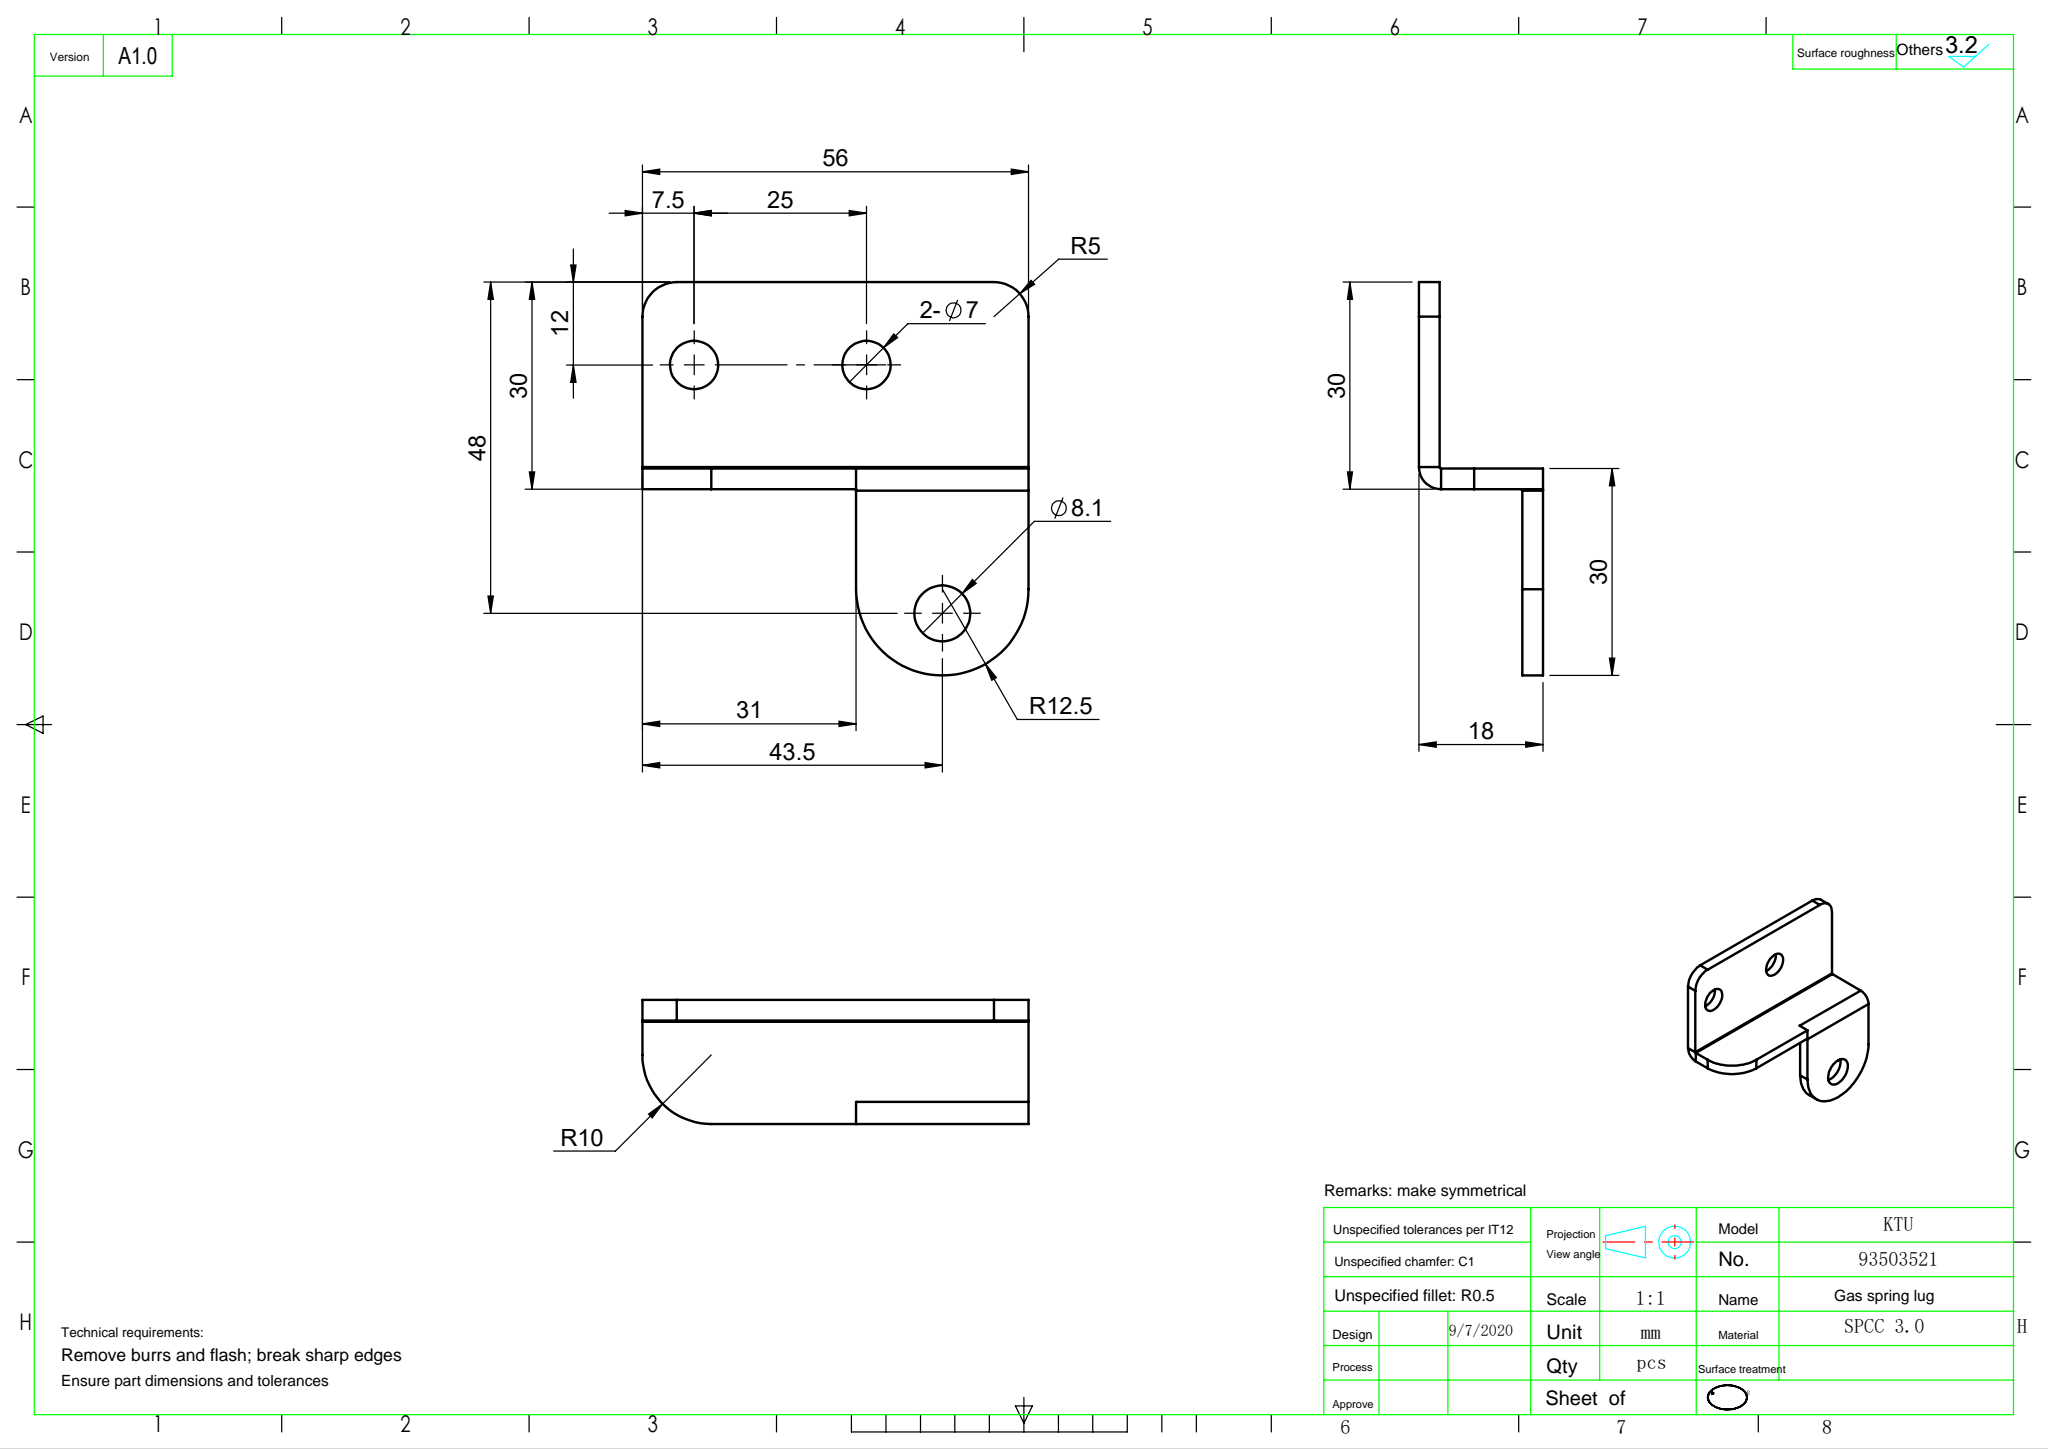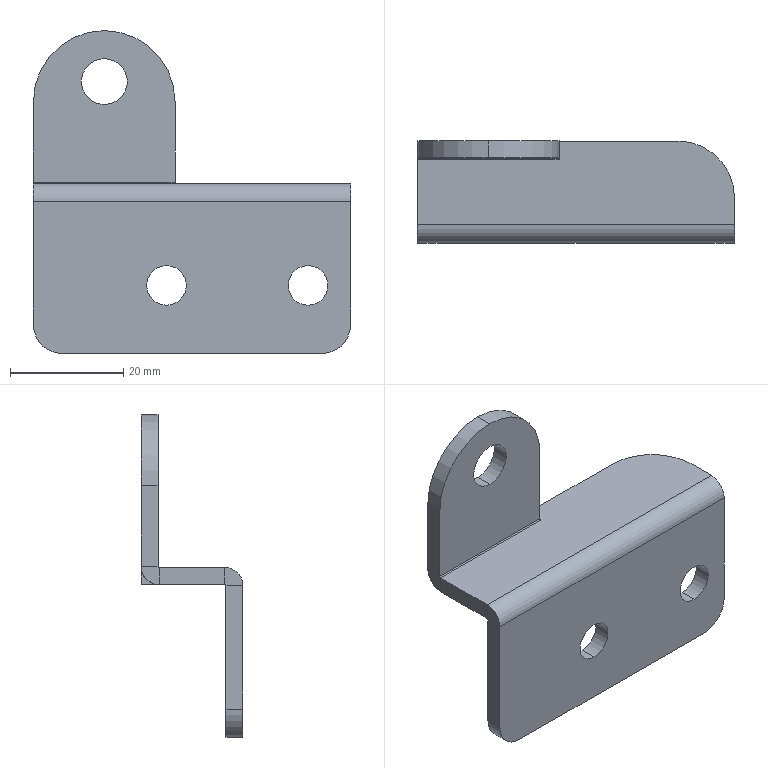Part | SolidWorks | features MirrorStock 1 | 1 solid | 34 faces | box 56 x 18 x 57 mm | volume 8724 mm3 | plane 19 | cylinder 15 | commonest cylinder face diameters 7 x4 0.4 x2 6.4 x2 8.1 x2 10 x2 25 x2
STEP:
#1=CARTESIAN_POINT('',(20.5,-9.,-18.5));
#2=VERTEX_POINT('',#1);
#3=CARTESIAN_POINT('',(20.5,-9.,-11.5));
#4=VERTEX_POINT('',#3);
#5=CARTESIAN_POINT('',(20.5,-9.,-15.));
#6=DIRECTION('',(0.,-1.,0.));
#7=DIRECTION('',(0.,0.,1.));
#8=AXIS2_PLACEMENT_3D('',#5,#6,#7);
#9=CIRCLE('',#8,3.5);
#10=EDGE_CURVE('',#2,#4,#9,.T.);
#11=ORIENTED_EDGE('',*,*,#10,.T.);
#12=CARTESIAN_POINT('',(20.5,-6.,-11.5));
#13=VERTEX_POINT('',#12);
#14=CARTESIAN_POINT('',(20.5,-9.001,-11.5));
#15=DIRECTION('',(0.,1.,0.));
#16=VECTOR('',#15,1000.);
#17=LINE('',#14,#16);
#18=EDGE_CURVE('',#4,#13,#17,.T.);
#19=ORIENTED_EDGE('',*,*,#18,.T.);
#20=CARTESIAN_POINT('',(20.5,-6.,-18.5));
#21=VERTEX_POINT('',#20);
#22=CARTESIAN_POINT('',(20.5,-6.,-15.));
#23=DIRECTION('',(0.,-1.,0.));
#24=DIRECTION('',(0.,0.,-1.));
#25=AXIS2_PLACEMENT_3D('',#22,#23,#24);
#26=CIRCLE('',#25,3.5);
#27=EDGE_CURVE('',#21,#13,#26,.T.);
#28=ORIENTED_EDGE('',*,*,#27,.F.);
#29=CARTESIAN_POINT('',(20.5,-9.001,-18.5));
#30=DIRECTION('',(0.,1.,0.));
#31=VECTOR('',#30,1000.);
#32=LINE('',#29,#31);
#33=EDGE_CURVE('',#2,#21,#32,.T.);
#34=ORIENTED_EDGE('',*,*,#33,.F.);
#35=EDGE_LOOP('',(#11,#19,#28,#34));
#36=FACE_OUTER_BOUND('',#35,.T.);
#37=CARTESIAN_POINT('',(20.5,-9.001,-15.));
#38=DIRECTION('',(0.,1.,0.));
#39=DIRECTION('',(0.,0.,-1.));
#40=AXIS2_PLACEMENT_3D('',#37,#38,#39);
#41=CYLINDRICAL_SURFACE('',#40,3.5);
#42=ADVANCED_FACE('',(#36),#41,.F.);
#43=CARTESIAN_POINT('',(-4.5,-9.,-18.5));
#44=VERTEX_POINT('',#43);
#45=CARTESIAN_POINT('',(-4.5,-9.,-11.5));
#46=VERTEX_POINT('',#45);
#47=CARTESIAN_POINT('',(-4.5,-9.,-15.));
#48=DIRECTION('',(0.,-1.,0.));
#49=DIRECTION('',(0.,0.,1.));
#50=AXIS2_PLACEMENT_3D('',#47,#48,#49);
#51=CIRCLE('',#50,3.5);
#52=EDGE_CURVE('',#44,#46,#51,.T.);
#53=ORIENTED_EDGE('',*,*,#52,.T.);
#54=CARTESIAN_POINT('',(-4.5,-6.,-11.5));
#55=VERTEX_POINT('',#54);
#56=CARTESIAN_POINT('',(-4.5,-9.001,-11.5));
#57=DIRECTION('',(0.,1.,0.));
#58=VECTOR('',#57,1000.);
#59=LINE('',#56,#58);
#60=EDGE_CURVE('',#46,#55,#59,.T.);
#61=ORIENTED_EDGE('',*,*,#60,.T.);
#62=CARTESIAN_POINT('',(-4.5,-6.,-18.5));
#63=VERTEX_POINT('',#62);
#64=CARTESIAN_POINT('',(-4.5,-6.,-15.));
#65=DIRECTION('',(0.,-1.,0.));
#66=DIRECTION('',(0.,0.,-1.));
#67=AXIS2_PLACEMENT_3D('',#64,#65,#66);
#68=CIRCLE('',#67,3.5);
#69=EDGE_CURVE('',#63,#55,#68,.T.);
#70=ORIENTED_EDGE('',*,*,#69,.F.);
#71=CARTESIAN_POINT('',(-4.5,-9.001,-18.5));
#72=DIRECTION('',(0.,1.,0.));
#73=VECTOR('',#72,1000.);
#74=LINE('',#71,#73);
#75=EDGE_CURVE('',#44,#63,#74,.T.);
#76=ORIENTED_EDGE('',*,*,#75,.F.);
#77=EDGE_LOOP('',(#53,#61,#70,#76));
#78=FACE_OUTER_BOUND('',#77,.T.);
#79=CARTESIAN_POINT('',(-4.5,-9.001,-15.));
#80=DIRECTION('',(0.,1.,0.));
#81=DIRECTION('',(0.,0.,-1.));
#82=AXIS2_PLACEMENT_3D('',#79,#80,#81);
#83=CYLINDRICAL_SURFACE('',#82,3.5);
#84=ADVANCED_FACE('',(#78),#83,.F.);
#85=CARTESIAN_POINT('',(-15.5,6.,25.05));
#86=VERTEX_POINT('',#85);
#87=CARTESIAN_POINT('',(-15.5,6.,16.95));
#88=VERTEX_POINT('',#87);
#89=CARTESIAN_POINT('',(-15.5,6.,21.));
#90=DIRECTION('',(0.,1.,0.));
#91=DIRECTION('',(0.,0.,-1.));
#92=AXIS2_PLACEMENT_3D('',#89,#90,#91);
#93=CIRCLE('',#92,4.05);
#94=EDGE_CURVE('',#86,#88,#93,.T.);
#95=ORIENTED_EDGE('',*,*,#94,.F.);
#96=CARTESIAN_POINT('',(-15.5,9.,25.05));
#97=VERTEX_POINT('',#96);
#98=CARTESIAN_POINT('',(-15.5,-9.001,25.05));
#99=DIRECTION('',(0.,1.,0.));
#100=VECTOR('',#99,1000.);
#101=LINE('',#98,#100);
#102=EDGE_CURVE('',#86,#97,#101,.T.);
#103=ORIENTED_EDGE('',*,*,#102,.T.);
#104=CARTESIAN_POINT('',(-15.5,9.,16.95));
#105=VERTEX_POINT('',#104);
#106=CARTESIAN_POINT('',(-15.5,9.,21.));
#107=DIRECTION('',(0.,-1.,0.));
#108=DIRECTION('',(0.,0.,-1.));
#109=AXIS2_PLACEMENT_3D('',#106,#107,#108);
#110=CIRCLE('',#109,4.05);
#111=EDGE_CURVE('',#105,#97,#110,.T.);
#112=ORIENTED_EDGE('',*,*,#111,.F.);
#113=CARTESIAN_POINT('',(-15.5,-9.001,16.95));
#114=DIRECTION('',(0.,1.,0.));
#115=VECTOR('',#114,1000.);
#116=LINE('',#113,#115);
#117=EDGE_CURVE('',#88,#105,#116,.T.);
#118=ORIENTED_EDGE('',*,*,#117,.F.);
#119=EDGE_LOOP('',(#95,#103,#112,#118));
#120=FACE_OUTER_BOUND('',#119,.T.);
#121=CARTESIAN_POINT('',(-15.5,-9.001,21.));
#122=DIRECTION('',(0.,1.,0.));
#123=DIRECTION('',(0.,0.,-1.));
#124=AXIS2_PLACEMENT_3D('',#121,#122,#123);
#125=CYLINDRICAL_SURFACE('',#124,4.05);
#126=ADVANCED_FACE('',(#120),#125,.F.);
#127=CARTESIAN_POINT('',(-3.,9.,17.5));
#128=VERTEX_POINT('',#127);
#129=CARTESIAN_POINT('',(-15.5,9.,30.));
#130=VERTEX_POINT('',#129);
#131=CARTESIAN_POINT('',(-15.5,9.,17.5));
#132=DIRECTION('',(0.,-1.,0.));
#133=DIRECTION('',(0.,0.,-1.));
#134=AXIS2_PLACEMENT_3D('',#131,#132,#133);
#135=CIRCLE('',#134,12.5);
#136=EDGE_CURVE('',#128,#130,#135,.T.);
#137=ORIENTED_EDGE('',*,*,#136,.T.);
#138=CARTESIAN_POINT('',(-15.5,6.,30.));
#139=VERTEX_POINT('',#138);
#140=CARTESIAN_POINT('',(-15.5,6.,30.));
#141=DIRECTION('',(0.,-1.,0.));
#142=VECTOR('',#141,1000.);
#143=LINE('',#140,#142);
#144=EDGE_CURVE('',#130,#139,#143,.T.);
#145=ORIENTED_EDGE('',*,*,#144,.T.);
#146=CARTESIAN_POINT('',(-3.,6.,17.5));
#147=VERTEX_POINT('',#146);
#148=CARTESIAN_POINT('',(-15.5,6.,17.5));
#149=DIRECTION('',(0.,1.,0.));
#150=DIRECTION('',(0.,0.,-1.));
#151=AXIS2_PLACEMENT_3D('',#148,#149,#150);
#152=CIRCLE('',#151,12.5);
#153=EDGE_CURVE('',#139,#147,#152,.T.);
#154=ORIENTED_EDGE('',*,*,#153,.T.);
#155=CARTESIAN_POINT('',(-3.,9.,17.5));
#156=DIRECTION('',(0.,1.,0.));
#157=VECTOR('',#156,1000.);
#158=LINE('',#155,#157);
#159=EDGE_CURVE('',#147,#128,#158,.T.);
#160=ORIENTED_EDGE('',*,*,#159,.T.);
#161=EDGE_LOOP('',(#137,#145,#154,#160));
#162=FACE_OUTER_BOUND('',#161,.T.);
#163=CARTESIAN_POINT('',(-15.5,6.,17.5));
#164=DIRECTION('',(0.,-1.,0.));
#165=DIRECTION('',(0.,0.,1.));
#166=AXIS2_PLACEMENT_3D('',#163,#164,#165);
#167=CYLINDRICAL_SURFACE('',#166,12.5);
#168=ADVANCED_FACE('',(#162),#167,.T.);
#169=ORIENTED_EDGE('',*,*,#144,.F.);
#170=CARTESIAN_POINT('',(-28.,9.,17.5));
#171=VERTEX_POINT('',#170);
#172=CARTESIAN_POINT('',(-15.5,9.,17.5));
#173=DIRECTION('',(0.,-1.,0.));
#174=DIRECTION('',(0.,0.,-1.));
#175=AXIS2_PLACEMENT_3D('',#172,#173,#174);
#176=CIRCLE('',#175,12.5);
#177=EDGE_CURVE('',#130,#171,#176,.T.);
#178=ORIENTED_EDGE('',*,*,#177,.T.);
#179=CARTESIAN_POINT('',(-28.,6.,17.5));
#180=VERTEX_POINT('',#179);
#181=CARTESIAN_POINT('',(-28.,9.,17.5));
#182=DIRECTION('',(0.,-1.,0.));
#183=VECTOR('',#182,1000.);
#184=LINE('',#181,#183);
#185=EDGE_CURVE('',#171,#180,#184,.T.);
#186=ORIENTED_EDGE('',*,*,#185,.T.);
#187=CARTESIAN_POINT('',(-15.5,6.,17.5));
#188=DIRECTION('',(0.,1.,0.));
#189=DIRECTION('',(0.,0.,-1.));
#190=AXIS2_PLACEMENT_3D('',#187,#188,#189);
#191=CIRCLE('',#190,12.5);
#192=EDGE_CURVE('',#180,#139,#191,.T.);
#193=ORIENTED_EDGE('',*,*,#192,.T.);
#194=EDGE_LOOP('',(#169,#178,#186,#193));
#195=FACE_OUTER_BOUND('',#194,.T.);
#196=CARTESIAN_POINT('',(-15.5,6.,17.5));
#197=DIRECTION('',(0.,-1.,0.));
#198=DIRECTION('',(0.,0.,1.));
#199=AXIS2_PLACEMENT_3D('',#196,#197,#198);
#200=CYLINDRICAL_SURFACE('',#199,12.5);
#201=ADVANCED_FACE('',(#195),#200,.T.);
#202=CARTESIAN_POINT('',(-3.,9.,3.));
#203=VERTEX_POINT('',#202);
#204=CARTESIAN_POINT('',(-3.,8.994,3.));
#205=VERTEX_POINT('',#204);
#206=CARTESIAN_POINT('',(-3.,9.,3.));
#207=DIRECTION('',(0.,-1.,0.));
#208=VECTOR('',#207,1000.);
#209=LINE('',#206,#208);
#210=EDGE_CURVE('',#203,#205,#209,.T.);
#211=ORIENTED_EDGE('',*,*,#210,.F.);
#212=CARTESIAN_POINT('',(-3.,9.,0.));
#213=VERTEX_POINT('',#212);
#214=CARTESIAN_POINT('',(-3.,9.,3.));
#215=DIRECTION('',(0.,0.,-1.));
#216=VECTOR('',#215,1000.);
#217=LINE('',#214,#216);
#218=EDGE_CURVE('',#203,#213,#217,.T.);
#219=ORIENTED_EDGE('',*,*,#218,.T.);
#220=CARTESIAN_POINT('',(-3.,5.8,0.));
#221=VERTEX_POINT('',#220);
#222=CARTESIAN_POINT('',(-3.,0.,0.));
#223=DIRECTION('',(0.,-1.,0.));
#224=VECTOR('',#223,1000.);
#225=LINE('',#222,#224);
#226=EDGE_CURVE('',#213,#221,#225,.T.);
#227=ORIENTED_EDGE('',*,*,#226,.T.);
#228=CARTESIAN_POINT('',(-3.,5.8,3.2));
#229=DIRECTION('',(-1.,0.,0.));
#230=DIRECTION('',(0.,0.,1.));
#231=AXIS2_PLACEMENT_3D('',#228,#229,#230);
#232=CIRCLE('',#231,3.2);
#233=EDGE_CURVE('',#205,#221,#232,.T.);
#234=ORIENTED_EDGE('',*,*,#233,.F.);
#235=EDGE_LOOP('',(#211,#219,#227,#234));
#236=FACE_OUTER_BOUND('',#235,.T.);
#237=CARTESIAN_POINT('',(-3.,9.,3.));
#238=DIRECTION('',(-1.,0.,0.));
#239=DIRECTION('',(0.,0.,-1.));
#240=AXIS2_PLACEMENT_3D('',#237,#238,#239);
#241=PLANE('',#240);
#242=ADVANCED_FACE('',(#236),#241,.T.);
#243=CARTESIAN_POINT('',(18.,9.,3.));
#244=VERTEX_POINT('',#243);
#245=CARTESIAN_POINT('',(28.,9.,3.));
#246=DIRECTION('',(-1.,0.,0.));
#247=VECTOR('',#246,1000.);
#248=LINE('',#245,#247);
#249=EDGE_CURVE('',#244,#203,#248,.T.);
#250=ORIENTED_EDGE('',*,*,#249,.T.);
#251=ORIENTED_EDGE('',*,*,#210,.T.);
#252=CARTESIAN_POINT('',(-3.,5.8,3.));
#253=VERTEX_POINT('',#252);
#254=CARTESIAN_POINT('',(-3.,9.,3.));
#255=DIRECTION('',(0.,-1.,0.));
#256=VECTOR('',#255,1000.);
#257=LINE('',#254,#256);
#258=EDGE_CURVE('',#205,#253,#257,.T.);
#259=ORIENTED_EDGE('',*,*,#258,.T.);
#260=CARTESIAN_POINT('',(-28.,5.8,3.));
#261=VERTEX_POINT('',#260);
#262=CARTESIAN_POINT('',(-3.,5.8,3.));
#263=DIRECTION('',(-1.,0.,0.));
#264=VECTOR('',#263,1000.);
#265=LINE('',#262,#264);
#266=EDGE_CURVE('',#253,#261,#265,.T.);
#267=ORIENTED_EDGE('',*,*,#266,.T.);
#268=CARTESIAN_POINT('',(-28.,-5.8,3.));
#269=VERTEX_POINT('',#268);
#270=CARTESIAN_POINT('',(-28.,-9.,3.));
#271=DIRECTION('',(0.,-1.,0.));
#272=VECTOR('',#271,1000.);
#273=LINE('',#270,#272);
#274=EDGE_CURVE('',#261,#269,#273,.T.);
#275=ORIENTED_EDGE('',*,*,#274,.T.);
#276=CARTESIAN_POINT('',(28.,-5.8,3.));
#277=VERTEX_POINT('',#276);
#278=CARTESIAN_POINT('',(28.,-5.8,3.));
#279=DIRECTION('',(-1.,0.,0.));
#280=VECTOR('',#279,1000.);
#281=LINE('',#278,#280);
#282=EDGE_CURVE('',#277,#269,#281,.T.);
#283=ORIENTED_EDGE('',*,*,#282,.F.);
#284=CARTESIAN_POINT('',(28.,-1.,3.));
#285=VERTEX_POINT('',#284);
#286=CARTESIAN_POINT('',(28.,-9.,3.));
#287=DIRECTION('',(0.,1.,0.));
#288=VECTOR('',#287,1000.);
#289=LINE('',#286,#288);
#290=EDGE_CURVE('',#277,#285,#289,.T.);
#291=ORIENTED_EDGE('',*,*,#290,.T.);
#292=CARTESIAN_POINT('',(18.,-1.,3.));
#293=DIRECTION('',(0.,0.,-1.));
#294=DIRECTION('',(1.,0.,0.));
#295=AXIS2_PLACEMENT_3D('',#292,#293,#294);
#296=CIRCLE('',#295,10.);
#297=EDGE_CURVE('',#244,#285,#296,.T.);
#298=ORIENTED_EDGE('',*,*,#297,.F.);
#299=EDGE_LOOP('',(#250,#251,#259,#267,#275,#283,#291,#298));
#300=FACE_OUTER_BOUND('',#299,.T.);
#301=CARTESIAN_POINT('',(0.,0.,3.));
#302=DIRECTION('',(0.,0.,-1.));
#303=DIRECTION('',(1.,0.,0.));
#304=AXIS2_PLACEMENT_3D('',#301,#302,#303);
#305=PLANE('',#304);
#306=ADVANCED_FACE('',(#300),#305,.F.);
#307=CARTESIAN_POINT('',(28.,-5.8,0.));
#308=VERTEX_POINT('',#307);
#309=CARTESIAN_POINT('',(28.,-1.,0.));
#310=VERTEX_POINT('',#309);
#311=CARTESIAN_POINT('',(28.,-9.,0.));
#312=DIRECTION('',(0.,1.,0.));
#313=VECTOR('',#312,1000.);
#314=LINE('',#311,#313);
#315=EDGE_CURVE('',#308,#310,#314,.T.);
#316=ORIENTED_EDGE('',*,*,#315,.F.);
#317=CARTESIAN_POINT('',(-28.,-5.8,0.));
#318=VERTEX_POINT('',#317);
#319=CARTESIAN_POINT('',(28.,-5.8,0.));
#320=DIRECTION('',(-1.,0.,0.));
#321=VECTOR('',#320,1000.);
#322=LINE('',#319,#321);
#323=EDGE_CURVE('',#308,#318,#322,.T.);
#324=ORIENTED_EDGE('',*,*,#323,.T.);
#325=CARTESIAN_POINT('',(-28.,5.8,0.));
#326=VERTEX_POINT('',#325);
#327=CARTESIAN_POINT('',(-28.,-9.,0.));
#328=DIRECTION('',(0.,-1.,0.));
#329=VECTOR('',#328,1000.);
#330=LINE('',#327,#329);
#331=EDGE_CURVE('',#326,#318,#330,.T.);
#332=ORIENTED_EDGE('',*,*,#331,.F.);
#333=CARTESIAN_POINT('',(-3.,5.8,0.));
#334=DIRECTION('',(-1.,0.,0.));
#335=VECTOR('',#334,1000.);
#336=LINE('',#333,#335);
#337=EDGE_CURVE('',#221,#326,#336,.T.);
#338=ORIENTED_EDGE('',*,*,#337,.F.);
#339=ORIENTED_EDGE('',*,*,#226,.F.);
#340=CARTESIAN_POINT('',(18.,9.,0.));
#341=VERTEX_POINT('',#340);
#342=CARTESIAN_POINT('',(28.,9.,0.));
#343=DIRECTION('',(-1.,0.,0.));
#344=VECTOR('',#343,1000.);
#345=LINE('',#342,#344);
#346=EDGE_CURVE('',#341,#213,#345,.T.);
#347=ORIENTED_EDGE('',*,*,#346,.F.);
#348=CARTESIAN_POINT('',(18.,-1.,0.));
#349=DIRECTION('',(0.,0.,1.));
#350=DIRECTION('',(1.,0.,0.));
#351=AXIS2_PLACEMENT_3D('',#348,#349,#350);
#352=CIRCLE('',#351,10.);
#353=EDGE_CURVE('',#310,#341,#352,.T.);
#354=ORIENTED_EDGE('',*,*,#353,.F.);
#355=EDGE_LOOP('',(#316,#324,#332,#338,#339,#347,#354));
#356=FACE_OUTER_BOUND('',#355,.T.);
#357=CARTESIAN_POINT('',(0.,0.,0.));
#358=DIRECTION('',(0.,0.,-1.));
#359=DIRECTION('',(1.,0.,0.));
#360=AXIS2_PLACEMENT_3D('',#357,#358,#359);
#361=PLANE('',#360);
#362=ADVANCED_FACE('',(#356),#361,.T.);
#363=ORIENTED_EDGE('',*,*,#346,.T.);
#364=ORIENTED_EDGE('',*,*,#218,.F.);
#365=ORIENTED_EDGE('',*,*,#249,.F.);
#366=CARTESIAN_POINT('',(18.,9.,3.));
#367=DIRECTION('',(0.,0.,1.));
#368=VECTOR('',#367,1000.);
#369=LINE('',#366,#368);
#370=EDGE_CURVE('',#341,#244,#369,.T.);
#371=ORIENTED_EDGE('',*,*,#370,.F.);
#372=EDGE_LOOP('',(#363,#364,#365,#371));
#373=FACE_OUTER_BOUND('',#372,.T.);
#374=CARTESIAN_POINT('',(28.,9.,3.));
#375=DIRECTION('',(0.,1.,0.));
#376=DIRECTION('',(-1.,0.,0.));
#377=AXIS2_PLACEMENT_3D('',#374,#375,#376);
#378=PLANE('',#377);
#379=ADVANCED_FACE('',(#373),#378,.T.);
#380=ORIENTED_EDGE('',*,*,#290,.F.);
#381=CARTESIAN_POINT('',(28.,-5.8,0.));
#382=DIRECTION('',(0.,0.,1.));
#383=VECTOR('',#382,1000.);
#384=LINE('',#381,#383);
#385=EDGE_CURVE('',#308,#277,#384,.T.);
#386=ORIENTED_EDGE('',*,*,#385,.F.);
#387=ORIENTED_EDGE('',*,*,#315,.T.);
#388=CARTESIAN_POINT('',(28.,-1.,3.));
#389=DIRECTION('',(0.,0.,-1.));
#390=VECTOR('',#389,1000.);
#391=LINE('',#388,#390);
#392=EDGE_CURVE('',#285,#310,#391,.T.);
#393=ORIENTED_EDGE('',*,*,#392,.F.);
#394=EDGE_LOOP('',(#380,#386,#387,#393));
#395=FACE_OUTER_BOUND('',#394,.T.);
#396=CARTESIAN_POINT('',(28.,-9.,3.));
#397=DIRECTION('',(1.,0.,0.));
#398=DIRECTION('',(0.,0.,1.));
#399=AXIS2_PLACEMENT_3D('',#396,#397,#398);
#400=PLANE('',#399);
#401=ADVANCED_FACE('',(#395),#400,.T.);
#402=CARTESIAN_POINT('',(-28.,5.8,3.));
#403=DIRECTION('',(0.,0.,-1.));
#404=VECTOR('',#403,1000.);
#405=LINE('',#402,#404);
#406=EDGE_CURVE('',#261,#326,#405,.T.);
#407=ORIENTED_EDGE('',*,*,#406,.T.);
#408=ORIENTED_EDGE('',*,*,#331,.T.);
#409=CARTESIAN_POINT('',(-28.,-5.8,0.));
#410=DIRECTION('',(0.,0.,1.));
#411=VECTOR('',#410,1000.);
#412=LINE('',#409,#411);
#413=EDGE_CURVE('',#318,#269,#412,.T.);
#414=ORIENTED_EDGE('',*,*,#413,.T.);
#415=ORIENTED_EDGE('',*,*,#274,.F.);
#416=EDGE_LOOP('',(#407,#408,#414,#415));
#417=FACE_OUTER_BOUND('',#416,.T.);
#418=CARTESIAN_POINT('',(-28.,-9.,3.));
#419=DIRECTION('',(-1.,0.,0.));
#420=DIRECTION('',(0.,0.,-1.));
#421=AXIS2_PLACEMENT_3D('',#418,#419,#420);
#422=PLANE('',#421);
#423=ADVANCED_FACE('',(#417),#422,.T.);
#424=CARTESIAN_POINT('',(-28.,-6.,-0.2));
#425=VERTEX_POINT('',#424);
#426=CARTESIAN_POINT('',(-28.,-9.,-0.2));
#427=VERTEX_POINT('',#426);
#428=CARTESIAN_POINT('',(-28.,-9.,-0.2));
#429=DIRECTION('',(0.,-1.,0.));
#430=VECTOR('',#429,1000.);
#431=LINE('',#428,#430);
#432=EDGE_CURVE('',#425,#427,#431,.T.);
#433=ORIENTED_EDGE('',*,*,#432,.T.);
#434=CARTESIAN_POINT('',(-28.,-5.8,-0.2));
#435=DIRECTION('',(1.,0.,0.));
#436=DIRECTION('',(0.,0.,1.));
#437=AXIS2_PLACEMENT_3D('',#434,#435,#436);
#438=CIRCLE('',#437,3.2);
#439=EDGE_CURVE('',#269,#427,#438,.T.);
#440=ORIENTED_EDGE('',*,*,#439,.F.);
#441=ORIENTED_EDGE('',*,*,#413,.F.);
#442=CARTESIAN_POINT('',(-28.,-5.8,-0.2));
#443=DIRECTION('',(1.,0.,0.));
#444=DIRECTION('',(0.,0.,1.));
#445=AXIS2_PLACEMENT_3D('',#442,#443,#444);
#446=CIRCLE('',#445,0.2);
#447=EDGE_CURVE('',#318,#425,#446,.T.);
#448=ORIENTED_EDGE('',*,*,#447,.T.);
#449=EDGE_LOOP('',(#433,#440,#441,#448));
#450=FACE_OUTER_BOUND('',#449,.T.);
#451=CARTESIAN_POINT('',(-28.,-5.8,-0.2));
#452=DIRECTION('',(-1.,0.,0.));
#453=DIRECTION('',(0.,0.,-1.));
#454=AXIS2_PLACEMENT_3D('',#451,#452,#453);
#455=PLANE('',#454);
#456=ADVANCED_FACE('',(#450),#455,.T.);
#457=CARTESIAN_POINT('',(28.,-6.,-0.2));
#458=VERTEX_POINT('',#457);
#459=CARTESIAN_POINT('',(28.,-5.8,-0.2));
#460=DIRECTION('',(-1.,0.,0.));
#461=DIRECTION('',(0.,0.,1.));
#462=AXIS2_PLACEMENT_3D('',#459,#460,#461);
#463=CIRCLE('',#462,0.2);
#464=EDGE_CURVE('',#458,#308,#463,.T.);
#465=ORIENTED_EDGE('',*,*,#464,.T.);
#466=ORIENTED_EDGE('',*,*,#385,.T.);
#467=CARTESIAN_POINT('',(28.,-9.,-0.2));
#468=VERTEX_POINT('',#467);
#469=CARTESIAN_POINT('',(28.,-5.8,-0.2));
#470=DIRECTION('',(-1.,0.,0.));
#471=DIRECTION('',(0.,0.,1.));
#472=AXIS2_PLACEMENT_3D('',#469,#470,#471);
#473=CIRCLE('',#472,3.2);
#474=EDGE_CURVE('',#468,#277,#473,.T.);
#475=ORIENTED_EDGE('',*,*,#474,.F.);
#476=CARTESIAN_POINT('',(28.,-6.,-0.2));
#477=DIRECTION('',(0.,-1.,0.));
#478=VECTOR('',#477,1000.);
#479=LINE('',#476,#478);
#480=EDGE_CURVE('',#458,#468,#479,.T.);
#481=ORIENTED_EDGE('',*,*,#480,.F.);
#482=EDGE_LOOP('',(#465,#466,#475,#481));
#483=FACE_OUTER_BOUND('',#482,.T.);
#484=CARTESIAN_POINT('',(28.,-5.8,-0.2));
#485=DIRECTION('',(-1.,0.,0.));
#486=DIRECTION('',(0.,0.,-1.));
#487=AXIS2_PLACEMENT_3D('',#484,#485,#486);
#488=PLANE('',#487);
#489=ADVANCED_FACE('',(#483),#488,.F.);
#490=ORIENTED_EDGE('',*,*,#282,.T.);
#491=ORIENTED_EDGE('',*,*,#439,.T.);
#492=CARTESIAN_POINT('',(0.,-9.,-0.2));
#493=DIRECTION('',(1.,0.,0.));
#494=VECTOR('',#493,1000.);
#495=LINE('',#492,#494);
#496=EDGE_CURVE('',#427,#468,#495,.T.);
#497=ORIENTED_EDGE('',*,*,#496,.T.);
#498=ORIENTED_EDGE('',*,*,#474,.T.);
#499=EDGE_LOOP('',(#490,#491,#497,#498));
#500=FACE_OUTER_BOUND('',#499,.T.);
#501=CARTESIAN_POINT('',(28.,-5.8,-0.2));
#502=DIRECTION('',(1.,0.,0.));
#503=DIRECTION('',(0.,-1.,0.));
#504=AXIS2_PLACEMENT_3D('',#501,#502,#503);
#505=CYLINDRICAL_SURFACE('',#504,3.2);
#506=ADVANCED_FACE('',(#500),#505,.T.);
#507=ORIENTED_EDGE('',*,*,#323,.F.);
#508=ORIENTED_EDGE('',*,*,#464,.F.);
#509=CARTESIAN_POINT('',(-28.,-6.,-0.2));
#510=DIRECTION('',(1.,0.,0.));
#511=VECTOR('',#510,1000.);
#512=LINE('',#509,#511);
#513=EDGE_CURVE('',#425,#458,#512,.T.);
#514=ORIENTED_EDGE('',*,*,#513,.F.);
#515=ORIENTED_EDGE('',*,*,#447,.F.);
#516=EDGE_LOOP('',(#507,#508,#514,#515));
#517=FACE_OUTER_BOUND('',#516,.T.);
#518=CARTESIAN_POINT('',(28.,-5.8,-0.2));
#519=DIRECTION('',(1.,0.,0.));
#520=DIRECTION('',(0.,-1.,0.));
#521=AXIS2_PLACEMENT_3D('',#518,#519,#520);
#522=CYLINDRICAL_SURFACE('',#521,0.2);
#523=ADVANCED_FACE('',(#517),#522,.F.);
#524=CARTESIAN_POINT('',(28.,-6.,-22.));
#525=VERTEX_POINT('',#524);
#526=CARTESIAN_POINT('',(28.,-6.,0.));
#527=DIRECTION('',(0.,0.,1.));
#528=VECTOR('',#527,1000.);
#529=LINE('',#526,#528);
#530=EDGE_CURVE('',#525,#458,#529,.T.);
#531=ORIENTED_EDGE('',*,*,#530,.T.);
#532=ORIENTED_EDGE('',*,*,#480,.T.);
#533=CARTESIAN_POINT('',(28.,-9.,-22.));
#534=VERTEX_POINT('',#533);
#535=CARTESIAN_POINT('',(28.,-9.,0.));
#536=DIRECTION('',(0.,0.,1.));
#537=VECTOR('',#536,1000.);
#538=LINE('',#535,#537);
#539=EDGE_CURVE('',#534,#468,#538,.T.);
#540=ORIENTED_EDGE('',*,*,#539,.F.);
#541=CARTESIAN_POINT('',(28.,-9.,-22.));
#542=DIRECTION('',(0.,-1.,0.));
#543=VECTOR('',#542,1000.);
#544=LINE('',#541,#543);
#545=EDGE_CURVE('',#525,#534,#544,.T.);
#546=ORIENTED_EDGE('',*,*,#545,.F.);
#547=EDGE_LOOP('',(#531,#532,#540,#546));
#548=FACE_OUTER_BOUND('',#547,.T.);
#549=CARTESIAN_POINT('',(28.,-9.,0.));
#550=DIRECTION('',(1.,0.,0.));
#551=DIRECTION('',(0.,0.,1.));
#552=AXIS2_PLACEMENT_3D('',#549,#550,#551);
#553=PLANE('',#552);
#554=ADVANCED_FACE('',(#548),#553,.T.);
#555=CARTESIAN_POINT('',(-28.,-9.,-22.));
#556=VERTEX_POINT('',#555);
#557=CARTESIAN_POINT('',(-28.,-9.,-27.));
#558=DIRECTION('',(0.,0.,-1.));
#559=VECTOR('',#558,1000.);
#560=LINE('',#557,#559);
#561=EDGE_CURVE('',#427,#556,#560,.T.);
#562=ORIENTED_EDGE('',*,*,#561,.F.);
#563=ORIENTED_EDGE('',*,*,#432,.F.);
#564=CARTESIAN_POINT('',(-28.,-6.,-22.));
#565=VERTEX_POINT('',#564);
#566=CARTESIAN_POINT('',(-28.,-6.,0.));
#567=DIRECTION('',(0.,0.,-1.));
#568=VECTOR('',#567,1000.);
#569=LINE('',#566,#568);
#570=EDGE_CURVE('',#425,#565,#569,.T.);
#571=ORIENTED_EDGE('',*,*,#570,.T.);
#572=CARTESIAN_POINT('',(-28.,-9.,-22.));
#573=DIRECTION('',(0.,1.,0.));
#574=VECTOR('',#573,1000.);
#575=LINE('',#572,#574);
#576=EDGE_CURVE('',#556,#565,#575,.T.);
#577=ORIENTED_EDGE('',*,*,#576,.F.);
#578=EDGE_LOOP('',(#562,#563,#571,#577));
#579=FACE_OUTER_BOUND('',#578,.T.);
#580=CARTESIAN_POINT('',(-28.,-9.,-27.));
#581=DIRECTION('',(-1.,0.,0.));
#582=DIRECTION('',(0.,0.,-1.));
#583=AXIS2_PLACEMENT_3D('',#580,#581,#582);
#584=PLANE('',#583);
#585=ADVANCED_FACE('',(#579),#584,.T.);
#586=ORIENTED_EDGE('',*,*,#10,.F.);
#587=CARTESIAN_POINT('',(20.5,-9.,-15.));
#588=DIRECTION('',(0.,-1.,0.));
#589=DIRECTION('',(0.,0.,1.));
#590=AXIS2_PLACEMENT_3D('',#587,#588,#589);
#591=CIRCLE('',#590,3.5);
#592=EDGE_CURVE('',#4,#2,#591,.T.);
#593=ORIENTED_EDGE('',*,*,#592,.F.);
#594=EDGE_LOOP('',(#586,#593));
#595=FACE_BOUND('',#594,.T.);
#596=ORIENTED_EDGE('',*,*,#52,.F.);
#597=CARTESIAN_POINT('',(-4.5,-9.,-15.));
#598=DIRECTION('',(0.,-1.,0.));
#599=DIRECTION('',(0.,0.,1.));
#600=AXIS2_PLACEMENT_3D('',#597,#598,#599);
#601=CIRCLE('',#600,3.5);
#602=EDGE_CURVE('',#46,#44,#601,.T.);
#603=ORIENTED_EDGE('',*,*,#602,.F.);
#604=EDGE_LOOP('',(#596,#603));
#605=FACE_BOUND('',#604,.T.);
#606=CARTESIAN_POINT('',(-23.,-9.,-27.));
#607=VERTEX_POINT('',#606);
#608=CARTESIAN_POINT('',(23.,-9.,-27.));
#609=VERTEX_POINT('',#608);
#610=CARTESIAN_POINT('',(28.,-9.,-27.));
#611=DIRECTION('',(1.,0.,0.));
#612=VECTOR('',#611,1000.);
#613=LINE('',#610,#612);
#614=EDGE_CURVE('',#607,#609,#613,.T.);
#615=ORIENTED_EDGE('',*,*,#614,.T.);
#616=CARTESIAN_POINT('',(23.,-9.,-22.));
#617=DIRECTION('',(0.,1.,0.));
#618=DIRECTION('',(0.,0.,1.));
#619=AXIS2_PLACEMENT_3D('',#616,#617,#618);
#620=CIRCLE('',#619,5.);
#621=EDGE_CURVE('',#534,#609,#620,.T.);
#622=ORIENTED_EDGE('',*,*,#621,.F.);
#623=ORIENTED_EDGE('',*,*,#539,.T.);
#624=ORIENTED_EDGE('',*,*,#496,.F.);
#625=ORIENTED_EDGE('',*,*,#561,.T.);
#626=CARTESIAN_POINT('',(-23.,-9.,-22.));
#627=DIRECTION('',(0.,1.,0.));
#628=DIRECTION('',(0.,0.,1.));
#629=AXIS2_PLACEMENT_3D('',#626,#627,#628);
#630=CIRCLE('',#629,5.);
#631=EDGE_CURVE('',#607,#556,#630,.T.);
#632=ORIENTED_EDGE('',*,*,#631,.F.);
#633=EDGE_LOOP('',(#615,#622,#623,#624,#625,#632));
#634=FACE_OUTER_BOUND('',#633,.T.);
#635=CARTESIAN_POINT('',(0.,-9.,0.));
#636=DIRECTION('',(0.,-1.,0.));
#637=DIRECTION('',(0.,0.,1.));
#638=AXIS2_PLACEMENT_3D('',#635,#636,#637);
#639=PLANE('',#638);
#640=ADVANCED_FACE('',(#595,#605,#634),#639,.T.);
#641=ORIENTED_EDGE('',*,*,#27,.T.);
#642=CARTESIAN_POINT('',(20.5,-6.,-15.));
#643=DIRECTION('',(0.,-1.,0.));
#644=DIRECTION('',(0.,0.,-1.));
#645=AXIS2_PLACEMENT_3D('',#642,#643,#644);
#646=CIRCLE('',#645,3.5);
#647=EDGE_CURVE('',#13,#21,#646,.T.);
#648=ORIENTED_EDGE('',*,*,#647,.T.);
#649=EDGE_LOOP('',(#641,#648));
#650=FACE_BOUND('',#649,.T.);
#651=ORIENTED_EDGE('',*,*,#69,.T.);
#652=CARTESIAN_POINT('',(-4.5,-6.,-15.));
#653=DIRECTION('',(0.,-1.,0.));
#654=DIRECTION('',(0.,0.,-1.));
#655=AXIS2_PLACEMENT_3D('',#652,#653,#654);
#656=CIRCLE('',#655,3.5);
#657=EDGE_CURVE('',#55,#63,#656,.T.);
#658=ORIENTED_EDGE('',*,*,#657,.T.);
#659=EDGE_LOOP('',(#651,#658));
#660=FACE_BOUND('',#659,.T.);
#661=ORIENTED_EDGE('',*,*,#570,.F.);
#662=ORIENTED_EDGE('',*,*,#513,.T.);
#663=ORIENTED_EDGE('',*,*,#530,.F.);
#664=CARTESIAN_POINT('',(23.,-6.,-27.));
#665=VERTEX_POINT('',#664);
#666=CARTESIAN_POINT('',(23.,-6.,-22.));
#667=DIRECTION('',(0.,-1.,0.));
#668=DIRECTION('',(0.,0.,1.));
#669=AXIS2_PLACEMENT_3D('',#666,#667,#668);
#670=CIRCLE('',#669,5.);
#671=EDGE_CURVE('',#665,#525,#670,.T.);
#672=ORIENTED_EDGE('',*,*,#671,.F.);
#673=CARTESIAN_POINT('',(-23.,-6.,-27.));
#674=VERTEX_POINT('',#673);
#675=CARTESIAN_POINT('',(0.,-6.,-27.));
#676=DIRECTION('',(1.,0.,0.));
#677=VECTOR('',#676,1000.);
#678=LINE('',#675,#677);
#679=EDGE_CURVE('',#674,#665,#678,.T.);
#680=ORIENTED_EDGE('',*,*,#679,.F.);
#681=CARTESIAN_POINT('',(-23.,-6.,-22.));
#682=DIRECTION('',(0.,-1.,0.));
#683=DIRECTION('',(0.,0.,1.));
#684=AXIS2_PLACEMENT_3D('',#681,#682,#683);
#685=CIRCLE('',#684,5.);
#686=EDGE_CURVE('',#565,#674,#685,.T.);
#687=ORIENTED_EDGE('',*,*,#686,.F.);
#688=EDGE_LOOP('',(#661,#662,#663,#672,#680,#687));
#689=FACE_OUTER_BOUND('',#688,.T.);
#690=CARTESIAN_POINT('',(0.,-6.,0.));
#691=DIRECTION('',(0.,-1.,0.));
#692=DIRECTION('',(0.,0.,1.));
#693=AXIS2_PLACEMENT_3D('',#690,#691,#692);
#694=PLANE('',#693);
#695=ADVANCED_FACE('',(#650,#660,#689),#694,.F.);
#696=ORIENTED_EDGE('',*,*,#679,.T.);
#697=CARTESIAN_POINT('',(23.,-9.,-27.));
#698=DIRECTION('',(0.,1.,0.));
#699=VECTOR('',#698,1000.);
#700=LINE('',#697,#699);
#701=EDGE_CURVE('',#609,#665,#700,.T.);
#702=ORIENTED_EDGE('',*,*,#701,.F.);
#703=ORIENTED_EDGE('',*,*,#614,.F.);
#704=CARTESIAN_POINT('',(-23.,-9.,-27.));
#705=DIRECTION('',(0.,-1.,0.));
#706=VECTOR('',#705,1000.);
#707=LINE('',#704,#706);
#708=EDGE_CURVE('',#674,#607,#707,.T.);
#709=ORIENTED_EDGE('',*,*,#708,.F.);
#710=EDGE_LOOP('',(#696,#702,#703,#709));
#711=FACE_OUTER_BOUND('',#710,.T.);
#712=CARTESIAN_POINT('',(28.,-9.,-27.));
#713=DIRECTION('',(0.,0.,-1.));
#714=DIRECTION('',(0.,-1.,0.));
#715=AXIS2_PLACEMENT_3D('',#712,#713,#714);
#716=PLANE('',#715);
#717=ADVANCED_FACE('',(#711),#716,.T.);
#718=CARTESIAN_POINT('',(-28.,6.,3.2));
#719=VERTEX_POINT('',#718);
#720=CARTESIAN_POINT('',(-28.,9.,3.2));
#721=VERTEX_POINT('',#720);
#722=CARTESIAN_POINT('',(-28.,9.,3.2));
#723=DIRECTION('',(0.,1.,0.));
#724=VECTOR('',#723,1000.);
#725=LINE('',#722,#724);
#726=EDGE_CURVE('',#719,#721,#725,.T.);
#727=ORIENTED_EDGE('',*,*,#726,.T.);
#728=CARTESIAN_POINT('',(-28.,5.8,3.2));
#729=DIRECTION('',(1.,0.,0.));
#730=DIRECTION('',(0.,0.,1.));
#731=AXIS2_PLACEMENT_3D('',#728,#729,#730);
#732=CIRCLE('',#731,3.2);
#733=EDGE_CURVE('',#326,#721,#732,.T.);
#734=ORIENTED_EDGE('',*,*,#733,.F.);
#735=ORIENTED_EDGE('',*,*,#406,.F.);
#736=CARTESIAN_POINT('',(-28.,5.8,3.2));
#737=DIRECTION('',(1.,0.,0.));
#738=DIRECTION('',(0.,0.,1.));
#739=AXIS2_PLACEMENT_3D('',#736,#737,#738);
#740=CIRCLE('',#739,0.2);
#741=EDGE_CURVE('',#261,#719,#740,.T.);
#742=ORIENTED_EDGE('',*,*,#741,.T.);
#743=EDGE_LOOP('',(#727,#734,#735,#742));
#744=FACE_OUTER_BOUND('',#743,.T.);
#745=CARTESIAN_POINT('',(-28.,5.8,3.2));
#746=DIRECTION('',(-1.,0.,0.));
#747=DIRECTION('',(0.,0.,-1.));
#748=AXIS2_PLACEMENT_3D('',#745,#746,#747);
#749=PLANE('',#748);
#750=ADVANCED_FACE('',(#744),#749,.T.);
#751=CARTESIAN_POINT('',(-3.,9.,3.2));
#752=VERTEX_POINT('',#751);
#753=CARTESIAN_POINT('',(-3.,5.8,3.2));
#754=DIRECTION('',(-1.,0.,0.));
#755=DIRECTION('',(0.,0.,1.));
#756=AXIS2_PLACEMENT_3D('',#753,#754,#755);
#757=CIRCLE('',#756,3.2);
#758=EDGE_CURVE('',#752,#205,#757,.T.);
#759=ORIENTED_EDGE('',*,*,#758,.F.);
#760=CARTESIAN_POINT('',(-3.,6.,3.2));
#761=VERTEX_POINT('',#760);
#762=CARTESIAN_POINT('',(-3.,6.,3.2));
#763=DIRECTION('',(0.,1.,0.));
#764=VECTOR('',#763,1000.);
#765=LINE('',#762,#764);
#766=EDGE_CURVE('',#761,#752,#765,.T.);
#767=ORIENTED_EDGE('',*,*,#766,.F.);
#768=CARTESIAN_POINT('',(-3.,5.8,3.2));
#769=DIRECTION('',(-1.,0.,0.));
#770=DIRECTION('',(0.,0.,1.));
#771=AXIS2_PLACEMENT_3D('',#768,#769,#770);
#772=CIRCLE('',#771,0.2);
#773=EDGE_CURVE('',#761,#253,#772,.T.);
#774=ORIENTED_EDGE('',*,*,#773,.T.);
#775=ORIENTED_EDGE('',*,*,#258,.F.);
#776=EDGE_LOOP('',(#759,#767,#774,#775));
#777=FACE_OUTER_BOUND('',#776,.T.);
#778=CARTESIAN_POINT('',(-3.,5.8,3.2));
#779=DIRECTION('',(-1.,0.,0.));
#780=DIRECTION('',(0.,0.,-1.));
#781=AXIS2_PLACEMENT_3D('',#778,#779,#780);
#782=PLANE('',#781);
#783=ADVANCED_FACE('',(#777),#782,.F.);
#784=ORIENTED_EDGE('',*,*,#337,.T.);
#785=ORIENTED_EDGE('',*,*,#733,.T.);
#786=CARTESIAN_POINT('',(0.,9.,3.2));
#787=DIRECTION('',(1.,0.,0.));
#788=VECTOR('',#787,1000.);
#789=LINE('',#786,#788);
#790=EDGE_CURVE('',#721,#752,#789,.T.);
#791=ORIENTED_EDGE('',*,*,#790,.T.);
#792=ORIENTED_EDGE('',*,*,#758,.T.);
#793=ORIENTED_EDGE('',*,*,#233,.T.);
#794=EDGE_LOOP('',(#784,#785,#791,#792,#793));
#795=FACE_OUTER_BOUND('',#794,.T.);
#796=CARTESIAN_POINT('',(-3.,5.8,3.2));
#797=DIRECTION('',(1.,0.,0.));
#798=DIRECTION('',(0.,1.,0.));
#799=AXIS2_PLACEMENT_3D('',#796,#797,#798);
#800=CYLINDRICAL_SURFACE('',#799,3.2);
#801=ADVANCED_FACE('',(#795),#800,.T.);
#802=ORIENTED_EDGE('',*,*,#266,.F.);
#803=ORIENTED_EDGE('',*,*,#773,.F.);
#804=CARTESIAN_POINT('',(-28.,6.,3.2));
#805=DIRECTION('',(1.,0.,0.));
#806=VECTOR('',#805,1000.);
#807=LINE('',#804,#806);
#808=EDGE_CURVE('',#719,#761,#807,.T.);
#809=ORIENTED_EDGE('',*,*,#808,.F.);
#810=ORIENTED_EDGE('',*,*,#741,.F.);
#811=EDGE_LOOP('',(#802,#803,#809,#810));
#812=FACE_OUTER_BOUND('',#811,.T.);
#813=CARTESIAN_POINT('',(-3.,5.8,3.2));
#814=DIRECTION('',(1.,0.,0.));
#815=DIRECTION('',(0.,1.,0.));
#816=AXIS2_PLACEMENT_3D('',#813,#814,#815);
#817=CYLINDRICAL_SURFACE('',#816,0.2);
#818=ADVANCED_FACE('',(#812),#817,.F.);
#819=CARTESIAN_POINT('',(-3.,6.,0.));
#820=DIRECTION('',(0.,0.,-1.));
#821=VECTOR('',#820,1000.);
#822=LINE('',#819,#821);
#823=EDGE_CURVE('',#147,#761,#822,.T.);
#824=ORIENTED_EDGE('',*,*,#823,.T.);
#825=ORIENTED_EDGE('',*,*,#766,.T.);
#826=CARTESIAN_POINT('',(-3.,9.,3.));
#827=DIRECTION('',(0.,0.,-1.));
#828=VECTOR('',#827,1000.);
#829=LINE('',#826,#828);
#830=EDGE_CURVE('',#128,#752,#829,.T.);
#831=ORIENTED_EDGE('',*,*,#830,.F.);
#832=ORIENTED_EDGE('',*,*,#159,.F.);
#833=EDGE_LOOP('',(#824,#825,#831,#832));
#834=FACE_OUTER_BOUND('',#833,.T.);
#835=CARTESIAN_POINT('',(-3.,9.,3.));
#836=DIRECTION('',(1.,0.,0.));
#837=DIRECTION('',(0.,1.,0.));
#838=AXIS2_PLACEMENT_3D('',#835,#836,#837);
#839=PLANE('',#838);
#840=ADVANCED_FACE('',(#834),#839,.T.);
#841=CARTESIAN_POINT('',(-28.,9.,30.));
#842=DIRECTION('',(0.,0.,1.));
#843=VECTOR('',#842,1000.);
#844=LINE('',#841,#843);
#845=EDGE_CURVE('',#721,#171,#844,.T.);
#846=ORIENTED_EDGE('',*,*,#845,.F.);
#847=ORIENTED_EDGE('',*,*,#726,.F.);
#848=CARTESIAN_POINT('',(-28.,6.,0.));
#849=DIRECTION('',(0.,0.,1.));
#850=VECTOR('',#849,1000.);
#851=LINE('',#848,#850);
#852=EDGE_CURVE('',#719,#180,#851,.T.);
#853=ORIENTED_EDGE('',*,*,#852,.T.);
#854=ORIENTED_EDGE('',*,*,#185,.F.);
#855=EDGE_LOOP('',(#846,#847,#853,#854));
#856=FACE_OUTER_BOUND('',#855,.T.);
#857=CARTESIAN_POINT('',(-28.,9.,30.));
#858=DIRECTION('',(-1.,0.,0.));
#859=DIRECTION('',(0.,0.,-1.));
#860=AXIS2_PLACEMENT_3D('',#857,#858,#859);
#861=PLANE('',#860);
#862=ADVANCED_FACE('',(#856),#861,.T.);
#863=ORIENTED_EDGE('',*,*,#111,.T.);
#864=CARTESIAN_POINT('',(-15.5,9.,21.));
#865=DIRECTION('',(0.,-1.,0.));
#866=DIRECTION('',(0.,0.,-1.));
#867=AXIS2_PLACEMENT_3D('',#864,#865,#866);
#868=CIRCLE('',#867,4.05);
#869=EDGE_CURVE('',#97,#105,#868,.T.);
#870=ORIENTED_EDGE('',*,*,#869,.T.);
#871=EDGE_LOOP('',(#863,#870));
#872=FACE_BOUND('',#871,.T.);
#873=ORIENTED_EDGE('',*,*,#830,.T.);
#874=ORIENTED_EDGE('',*,*,#790,.F.);
#875=ORIENTED_EDGE('',*,*,#845,.T.);
#876=ORIENTED_EDGE('',*,*,#177,.F.);
#877=ORIENTED_EDGE('',*,*,#136,.F.);
#878=EDGE_LOOP('',(#873,#874,#875,#876,#877));
#879=FACE_OUTER_BOUND('',#878,.T.);
#880=CARTESIAN_POINT('',(0.,9.,0.));
#881=DIRECTION('',(0.,1.,0.));
#882=DIRECTION('',(0.,0.,-1.));
#883=AXIS2_PLACEMENT_3D('',#880,#881,#882);
#884=PLANE('',#883);
#885=ADVANCED_FACE('',(#872,#879),#884,.T.);
#886=CARTESIAN_POINT('',(-15.5,6.,21.));
#887=DIRECTION('',(0.,1.,0.));
#888=DIRECTION('',(0.,0.,-1.));
#889=AXIS2_PLACEMENT_3D('',#886,#887,#888);
#890=CIRCLE('',#889,4.05);
#891=EDGE_CURVE('',#88,#86,#890,.T.);
#892=ORIENTED_EDGE('',*,*,#891,.T.);
#893=ORIENTED_EDGE('',*,*,#94,.T.);
#894=EDGE_LOOP('',(#892,#893));
#895=FACE_BOUND('',#894,.T.);
#896=ORIENTED_EDGE('',*,*,#852,.F.);
#897=ORIENTED_EDGE('',*,*,#808,.T.);
#898=ORIENTED_EDGE('',*,*,#823,.F.);
#899=ORIENTED_EDGE('',*,*,#153,.F.);
#900=ORIENTED_EDGE('',*,*,#192,.F.);
#901=EDGE_LOOP('',(#896,#897,#898,#899,#900));
#902=FACE_OUTER_BOUND('',#901,.T.);
#903=CARTESIAN_POINT('',(0.,6.,0.));
#904=DIRECTION('',(0.,1.,0.));
#905=DIRECTION('',(0.,0.,-1.));
#906=AXIS2_PLACEMENT_3D('',#903,#904,#905);
#907=PLANE('',#906);
#908=ADVANCED_FACE('',(#895,#902),#907,.F.);
#909=ORIENTED_EDGE('',*,*,#102,.F.);
#910=ORIENTED_EDGE('',*,*,#891,.F.);
#911=ORIENTED_EDGE('',*,*,#117,.T.);
#912=ORIENTED_EDGE('',*,*,#869,.F.);
#913=EDGE_LOOP('',(#909,#910,#911,#912));
#914=FACE_OUTER_BOUND('',#913,.T.);
#915=CARTESIAN_POINT('',(-15.5,-9.001,21.));
#916=DIRECTION('',(0.,1.,0.));
#917=DIRECTION('',(0.,0.,-1.));
#918=AXIS2_PLACEMENT_3D('',#915,#916,#917);
#919=CYLINDRICAL_SURFACE('',#918,4.05);
#920=ADVANCED_FACE('',(#914),#919,.F.);
#921=ORIENTED_EDGE('',*,*,#60,.F.);
#922=ORIENTED_EDGE('',*,*,#602,.T.);
#923=ORIENTED_EDGE('',*,*,#75,.T.);
#924=ORIENTED_EDGE('',*,*,#657,.F.);
#925=EDGE_LOOP('',(#921,#922,#923,#924));
#926=FACE_OUTER_BOUND('',#925,.T.);
#927=CARTESIAN_POINT('',(-4.5,-9.001,-15.));
#928=DIRECTION('',(0.,1.,0.));
#929=DIRECTION('',(0.,0.,-1.));
#930=AXIS2_PLACEMENT_3D('',#927,#928,#929);
#931=CYLINDRICAL_SURFACE('',#930,3.5);
#932=ADVANCED_FACE('',(#926),#931,.F.);
#933=ORIENTED_EDGE('',*,*,#18,.F.);
#934=ORIENTED_EDGE('',*,*,#592,.T.);
#935=ORIENTED_EDGE('',*,*,#33,.T.);
#936=ORIENTED_EDGE('',*,*,#647,.F.);
#937=EDGE_LOOP('',(#933,#934,#935,#936));
#938=FACE_OUTER_BOUND('',#937,.T.);
#939=CARTESIAN_POINT('',(20.5,-9.001,-15.));
#940=DIRECTION('',(0.,1.,0.));
#941=DIRECTION('',(0.,0.,-1.));
#942=AXIS2_PLACEMENT_3D('',#939,#940,#941);
#943=CYLINDRICAL_SURFACE('',#942,3.5);
#944=ADVANCED_FACE('',(#938),#943,.F.);
#945=ORIENTED_EDGE('',*,*,#297,.T.);
#946=ORIENTED_EDGE('',*,*,#392,.T.);
#947=ORIENTED_EDGE('',*,*,#353,.T.);
#948=ORIENTED_EDGE('',*,*,#370,.T.);
#949=EDGE_LOOP('',(#945,#946,#947,#948));
#950=FACE_OUTER_BOUND('',#949,.T.);
#951=CARTESIAN_POINT('',(18.,-1.,3.));
#952=DIRECTION('',(0.,0.,-1.));
#953=DIRECTION('',(1.,0.,0.));
#954=AXIS2_PLACEMENT_3D('',#951,#952,#953);
#955=CYLINDRICAL_SURFACE('',#954,10.);
#956=ADVANCED_FACE('',(#950),#955,.T.);
#957=ORIENTED_EDGE('',*,*,#631,.T.);
#958=ORIENTED_EDGE('',*,*,#576,.T.);
#959=ORIENTED_EDGE('',*,*,#686,.T.);
#960=ORIENTED_EDGE('',*,*,#708,.T.);
#961=EDGE_LOOP('',(#957,#958,#959,#960));
#962=FACE_OUTER_BOUND('',#961,.T.);
#963=CARTESIAN_POINT('',(-23.,-9.,-22.));
#964=DIRECTION('',(0.,1.,0.));
#965=DIRECTION('',(0.,0.,-1.));
#966=AXIS2_PLACEMENT_3D('',#963,#964,#965);
#967=CYLINDRICAL_SURFACE('',#966,5.);
#968=ADVANCED_FACE('',(#962),#967,.T.);
#969=ORIENTED_EDGE('',*,*,#621,.T.);
#970=ORIENTED_EDGE('',*,*,#701,.T.);
#971=ORIENTED_EDGE('',*,*,#671,.T.);
#972=ORIENTED_EDGE('',*,*,#545,.T.);
#973=EDGE_LOOP('',(#969,#970,#971,#972));
#974=FACE_OUTER_BOUND('',#973,.T.);
#975=CARTESIAN_POINT('',(23.,-9.,-22.));
#976=DIRECTION('',(0.,1.,0.));
#977=DIRECTION('',(0.,0.,-1.));
#978=AXIS2_PLACEMENT_3D('',#975,#976,#977);
#979=CYLINDRICAL_SURFACE('',#978,5.);
#980=ADVANCED_FACE('',(#974),#979,.T.);
#981=CLOSED_SHELL('',(#42,#84,#126,#168,#201,#242,#306,#362,#379,#401,#423,#456,#489,#506,#523,#554,#585,#640,#695,#717,#750,#783,#801,#818,#840,#862,#885,#908,#920,#932,#944,#956,#968,#980));
#982=MANIFOLD_SOLID_BREP('',#981);
#983=CARTESIAN_POINT('',(0.,0.,0.));
#984=DIRECTION('',(0.,0.,1.));
#985=DIRECTION('',(1.,0.,0.));
#986=AXIS2_PLACEMENT_3D('',#983,#984,#985);
#987=(LENGTH_UNIT()NAMED_UNIT(*)SI_UNIT(.MILLI.,.METRE.));
#988=UNCERTAINTY_MEASURE_WITH_UNIT(LENGTH_MEASURE(0.00001),#987,'','');
#989=(NAMED_UNIT(*)PLANE_ANGLE_UNIT()SI_UNIT($,.RADIAN.));
#990=(NAMED_UNIT(*)SI_UNIT($,.STERADIAN.)SOLID_ANGLE_UNIT());
#991=(GEOMETRIC_REPRESENTATION_CONTEXT(3)GLOBAL_UNCERTAINTY_ASSIGNED_CONTEXT((#988))GLOBAL_UNIT_ASSIGNED_CONTEXT((#987,#989,#990))REPRESENTATION_CONTEXT('',''));
#992=ADVANCED_BREP_SHAPE_REPRESENTATION('',(#982,#986),#991);